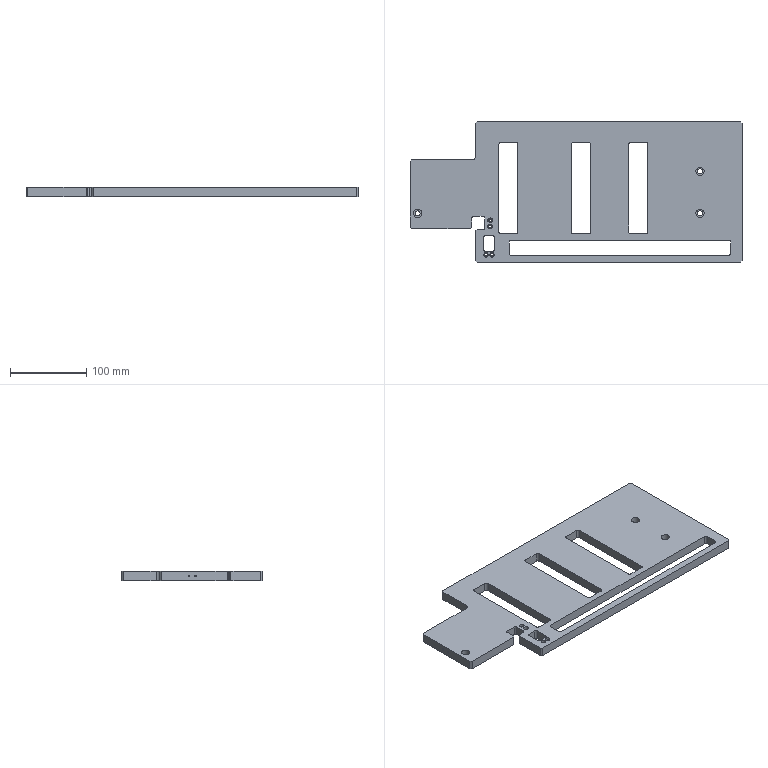NC program | NX | posted with a generic post | part box 435 x 184 x 12 mm
Whole program:
N10 G17 G21 G94 G90
(DRILLING_COPY_1_COPY , TOOL : D6A45)
N12 T01 M6
N14 G54
N16 G17 G0 G90 X132.5 Y-8. S5000 M3
N18 G43 Z30. H1
N20 G94 G81 G98 Z-2.1 F350. R3.
N22 X202.5
N24 G80
N26 G0 X202.5 Y-8. Z30.
N28 M5
(DRILLING_COPY_1_COPY_COPY_1_COPY_1 , TOOL : 3.3ZT)
N30 T17 M6
N32 G54
N34 G17 G0 G90 X132.5 Y-8. S2785 M3
N36 G43 Z30. H17
N38 G94 G83 G98 Z-13.961 F200. Q2. R3.
N40 X202.5
N42 G80
N44 G0 X202.5 Y-8. Z30.
N46 M5
(PLANAR_MILL_COPY_COPY_COPY_COPY_COPY_COPY_1_COPY_COPY_COPY , TOOL : D6A45)
N48 T01 M6
N50 G54
N52 G17 G0 G90 X209.35 Y-28.866 S9500 M3
N54 G43 Z30. H1
N56 Z0.5
N58 G94 G1 Z-1. F1250.
N60 G3 X209.85 Y-28. R1.
N62 X207.5 Y-25.65 R2.35
N64 X209.85 Y-28. R-2.35
N66 X209.35 Y-27.134 R1.
N68 G1 Z0.5
N70 G0 Z30.
N72 X202.971 Y-8.433
N74 Z0.5
N76 G1 Z-1.
N78 G3 X203.221 Y-8. R0.5
N80 X202.5 Y-7.279 R0.721
N82 X203.221 Y-8. R-0.721
N84 X202.971 Y-7.567 R0.5
N86 G1 Z0.5
N88 G0 Z30.
N90 X132.067 Y-8.471
N92 Z0.5
N94 G1 Z-1.
N96 G3 X132.5 Y-8.721 R0.5
N98 X133.221 Y-8. R0.721
N100 X132.5 Y-8.721 R-0.721
N102 X132.933 Y-8.471 R0.5
N104 G1 Z0.5
N106 G0 Z30.
N108 X112.067 Y-45.6
N110 Z0.5
N112 G1 Z-1.
N114 G3 X112.5 Y-45.85 R0.5
N116 X113.35 Y-45. R0.85
N118 X112.5 Y-45.85 R-0.85
N120 X112.933 Y-45.6 R0.5
N122 G1 Z0.5
N124 G0 Z30.
N126 X109.567 Y-83.1
N128 Z0.5
N130 G1 Z-1.
N132 G3 X110. Y-83.35 R0.5
N134 X110.85 Y-82.5 R0.85
N136 X110. Y-83.35 R-0.85
N138 X110.433 Y-83.1 R0.5
N140 G1 Z0.5
N142 G0 Z30.
N144 X117.567
N146 Z0.5
N148 G1 Z-1.
N150 G3 X118. Y-83.35 R0.5
N152 X118.85 Y-82.5 R0.85
N154 X118. Y-83.35 R-0.85
N156 X118.433 Y-83.1 R0.5
N158 G1 Z0.5
N160 G0 Z30.
N162 X120.1 Y-68.366
N164 Z0.5
N166 G1 Z-1.
N168 G3 X120.6 Y-67.5 R1.
N170 G1 Y-60.
N172 G3 X119. Y-58.4 R1.6
N174 G1 X109.
N176 G3 X107.4 Y-60. R1.6
N178 G1 Y-75.
N180 G3 X109. Y-76.6 R1.6
N182 G1 X119.
N184 G3 X120.6 Y-75. R1.6
N186 G1 Y-67.5
N188 G3 X120.1 Y-66.634 R1.
N190 G1 Z0.5
N192 G0 Z30.
N194 X112.067 Y-37.6
N196 Z0.5
N198 G1 Z-1.
N200 G3 X112.5 Y-37.85 R0.5
N202 X113.35 Y-37. R0.85
N204 X112.5 Y-37.85 R-0.85
N206 X112.933 Y-37.6 R0.5
N208 G1 Z0.5
N210 G0 Z30.
N212 X99.6 Y4.134
N214 Z0.5
N216 G1 Z-1.
N218 G3 X100.1 Y5. R1.
N220 G1 Y62.
N222 G3 X98. Y64.1 R2.1
N224 G1 X79.
N226 G3 X76.9 Y62. R2.1
N228 G1 Y-52.
N230 G3 X79. Y-54.1 R2.1
N232 G1 X98.
N234 G3 X100.1 Y-52. R2.1
N236 G1 Y5.
N238 G3 X99.6 Y5.866 R1.
N240 G1 Z0.5
N242 G0 Z30.
N244 X4.6 Y4.134
N246 Z0.5
N248 G1 Z-1.
N250 G3 X5.1 Y5. R1.
N252 G1 Y62.5
N254 G3 X3.5 Y64.1 R1.6
N256 G1 X-16.5
N258 G3 X-18.1 Y62.5 R1.6
N260 G1 Y-52.5
N262 G3 X-16.5 Y-54.1 R1.6
N264 G1 X3.5
N266 G3 X5.1 Y-52.5 R1.6
N268 G1 Y5.
N270 G3 X4.6 Y5.866 R1.
N272 G1 Z0.5
N274 G0 Z30.
N276 X-43.866 Y93.4
N278 Z0.5
N280 G1 Z-1.
N282 G3 X-43. Y92.9 R1.
N284 G1 X129.5
N286 G2 X130.136 Y92.636 R0.9
N288 G1 X132.136 Y90.636
N290 G2 X132.4 Y90. R0.9
N292 G1 Y47.
N294 G3 X136.5 Y42.9 R4.1
N296 G1 X215.5
N298 G2 X216.136 Y42.636 R0.9
N300 G1 X218.136 Y40.636
N302 G2 X218.4 Y40. R0.9
N304 G1 Y-46.
N306 G2 X218.136 Y-46.636 R0.9
N308 G1 X216.136 Y-48.636
N310 G2 X215.5 Y-48.9 R0.9
N312 G1 X138.5
N314 G2 X137.864 Y-48.636 R0.9
N316 G1 X135.864 Y-46.636
N318 G2 X135.6 Y-46. R0.9
N320 G1 Y-34.
N322 G3 X134.5 Y-32.9 R1.1
N324 G1 X121.5
N326 G3 X120.4 Y-34. R1.1
N328 G1 Y-47.
N330 G3 X121.5 Y-48.1 R1.1
N332 G1 X129.5
N334 G2 X130.136 Y-48.364 R0.9
N336 G1 X132.136 Y-50.364
N338 G2 X132.4 Y-51. R0.9
N340 G1 Y-90.
N342 G2 X132.136 Y-90.636 R0.9
N344 G1 X130.136 Y-92.636
N346 G2 X129.5 Y-92.9 R0.9
N348 G1 X-215.5
N350 G2 X-216.136 Y-92.636 R0.9
N352 G1 X-218.136 Y-90.636
N354 G2 X-218.4 Y-90. R0.9
N356 G1 Y90.
N358 G2 X-218.136 Y90.636 R0.9
N360 G1 X-216.136 Y92.636
N362 G2 X-215.5 Y92.9 R0.9
N364 G1 X-43.
N366 G3 X-42.134 Y93.4 R1.
N368 G1 Z0.5
N370 G0 Z30.
N372 X-58.366 Y-81.6
N374 Z0.5
N376 G1 Z-1.
N378 G3 X-57.5 Y-82.1 R1.
N380 G1 X85.
N382 G3 X86.6 Y-80.5 R1.6
N384 G1 Y-65.5
N386 G3 X85. Y-63.9 R1.6
N388 G1 X-200.
N390 G3 X-201.6 Y-65.5 R1.6
N392 G1 Y-80.5
N394 G3 X-200. Y-82.1 R1.6
N396 G1 X-57.5
N398 G3 X-56.634 Y-81.6 R1.
N400 G1 Z0.5
N402 G0 Z30.
N404 X-70.4 Y4.134
N406 Z0.5
N408 G1 Z-1.
N410 G3 X-69.9 Y5. R1.
N412 G1 Y62.5
N414 G3 X-71.5 Y64.1 R1.6
N416 G1 X-91.5
N418 G3 X-93.1 Y62.5 R1.6
N420 G1 Y-52.5
N422 G3 X-91.5 Y-54.1 R1.6
N424 G1 X-71.5
N426 G3 X-69.9 Y-52.5 R1.6
N428 G1 Y5.
N430 G3 X-70.4 Y5.866 R1.
N432 G1 Z0.5
N434 G0 Z30.
N436 X-164.35 Y27.866
N438 Z0.5
N440 G1 Z-1.
N442 G3 X-164.85 Y27. R1.
N444 X-162.5 Y24.65 R2.35
N446 X-164.85 Y27. R-2.35
N448 X-164.35 Y26.134 R1.
N450 G1 Z0.5
N452 G0 Z30.
N454 Y-27.134
N456 Z0.5
N458 G1 Z-1.
N460 G3 X-164.85 Y-28. R1.
N462 X-162.5 Y-30.35 R2.35
N464 X-164.85 Y-28. R-2.35
N466 X-164.35 Y-28.866 R1.
N468 G1 Z0.5
N470 G0 Z30.
N472 M5
N474 M2